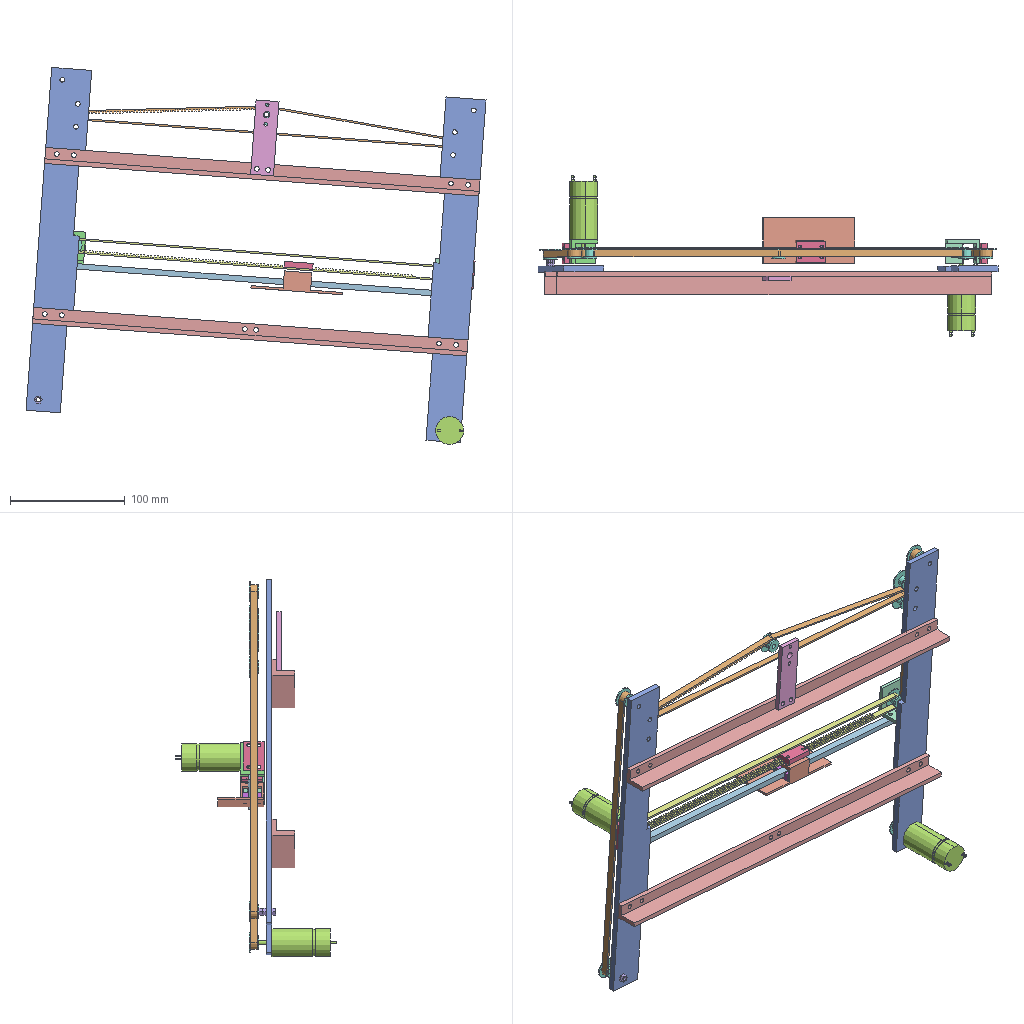Assembly | SolidWorks | 14 different items | 31 placed | box 401 x 140 x 329 mm
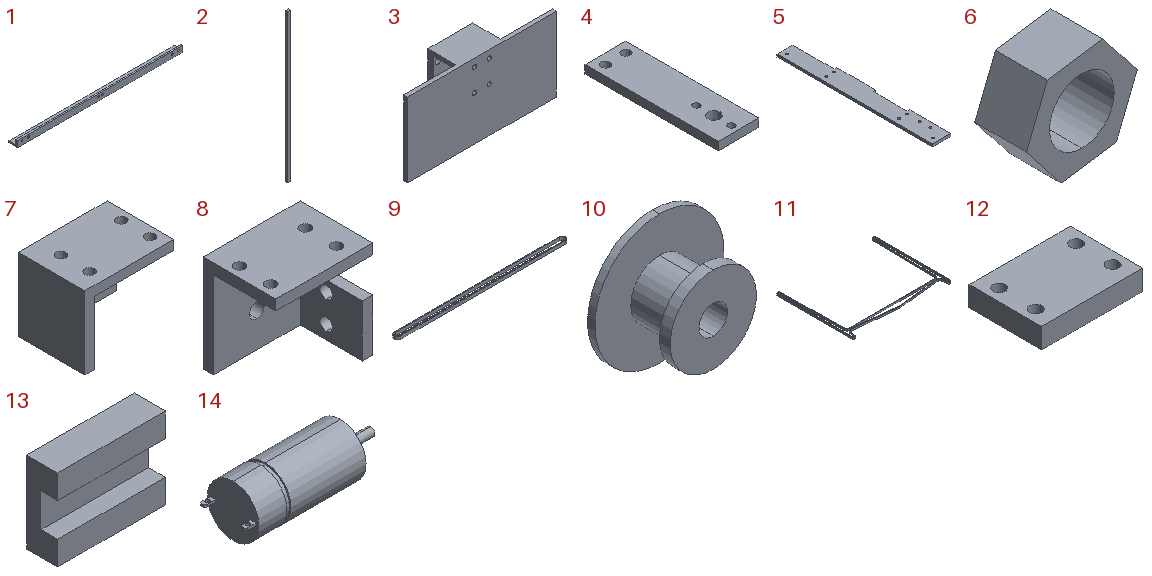Parts list (item | quantity | size | volume | features):
1 | x2 | 380 x 20 x 14 mm | 45267 mm3 | features Extrusion 1, ICE 1
2 | x1 | 7 x 4.8 x 340 mm | 11424 mm3 | features ICE 2, Extrusion 1, LPattern 1
3 | x1 | 80 x 17 x 40 mm | 8877 mm3 | features ICE 3, Extrusion 1
4 | x1 | 20 x 65 x 4 mm | 4912 mm3 | features Extrusion 1
5 | x2 | 35 x 300 x 5 mm | 48321 mm3 | features Extrusion 1
6 | x3 | 6.858 x 3.2 x 6.431 mm | 59.554 mm3 | features Extrusion 1
7 | x1 | 28 x 21 x 23 mm | 4355 mm3 | features ICE 2, Extrusion 1
8 | x1 | 28 x 21 x 28 mm | 4495 mm3 | features ICE 2, Extrusion 1
9 | x1 | 338 x 13 x 6 mm | 7437 mm3 | features Extrusion 1, ICE 1, LPattern 1
10 | x11 | 18 x 8.5 x 18 mm | 618.894 mm3 | features Revolution 1
11 | x1 | 372 x 292 x 6 mm | 17336 mm3 | features Extrusion 1, ICE 1, LPattern 1
12 | x3 | 25 x 18 x 5 mm | 2109 mm3 | features Extrusion 1
13 | x1 | 22.5 x 6.5 x 17 mm | 1885 mm3 | features Extrusion 1, ICE 1
14 | x2 | 70.5 x 24.5 x 24.5 mm | 24091 mm3 | features ICE 4, Extrusion 1, Fillet 1, RevCut 1
Mates (type | each side: item.copy, entity, surface, feature):
Concentric | 5.1 face cylinder Boss-Extrude1 | 10.1 face cylinder Revolve1
Concentric | 5.1 face cylinder Boss-Extrude1 | 10.2 face cylinder Revolve1
Concentric | 5.1 face cylinder Boss-Extrude1 | 10.3 face cylinder Revolve1
Concentric | 5.1 face cylinder Boss-Extrude1 | 10.4 face cylinder Revolve1
Coincident | 10.5 face plane Revolve1 | 10.3 face plane Revolve1
Concentric | 10.1 face cylinder Revolve1 | 11.1 face cylinder Boss-Extrude1
Concentric | 10.6 face cylinder Revolve1 | 11.1 face cylinder Boss-Extrude1
Coincident | 10.6 face plane Revolve1 | 11.1 face plane Boss-Extrude1
Concentric | 5.1 face cylinder Boss-Extrude1 | 6.1 face cylinder Boss-Extrude1
Coincident | 10.1 face plane Revolve1 | 6.1 face plane Boss-Extrude1
Coincident | 10.1 face plane Revolve1 | 11.1 face plane Boss-Extrude1
Coincident | 10.1 face plane Revolve1 | 10.4 face plane Revolve1
Coincident | 10.4 face plane Revolve1 | 10.3 face plane Revolve1
Coincident | 10.2 face plane Revolve1 | 10.4 face plane Revolve1
Coincident | 5.1 face plane Boss-Extrude1 | 6.2 face plane Boss-Extrude1
Coincident | 6.1 face plane Boss-Extrude1 | 6.3 face plane Boss-Extrude1
Coincident | 5.1 face plane Boss-Extrude1 | 6.3 face plane Boss-Extrude1
Coincident | 11.1 face plane Boss-Extrude1 | 12.1 face plane Boss-Extrude1
DistanceDim | 12.1 face plane Boss-Extrude1 | 11.1 face plane Boss-Extrude1
Coincident | 11.1 face plane Boss-Extrude1 | 8.1 face plane Boss-Extrude1
Concentric | 12.1 face cylinder Boss-Extrude1 | 8.1 face cylinder Boss-Extrude1 | 2 times
Concentric | 10.7 face cylinder Revolve1 | 8.1 face cylinder Boss-Extrude2
Parallel | 9.1 face plane Boss-Extrude1 | 8.1 face plane Boss-Extrude3
Concentric | 7.1 face cylinder Boss-Extrude2 | 10.8 face cylinder Revolve1
Coincident | 10.7 face plane Revolve1 | 9.1 face plane Boss-Extrude1
Coincident | 10.8 face plane Revolve1 | 9.1 face plane Boss-Extrude1
DistanceDim | 12.2 face plane Boss-Extrude1 | 7.1 face plane Boss-Extrude1
Concentric | 7.1 face cylinder Boss-Extrude1 | 12.2 face cylinder Boss-Extrude1 | 2 times
DistanceDim | 2.1 face plane Boss-Extrude1 | 7.1 face plane Boss-Extrude2
DistanceDim | 8.1 face plane Boss-Extrude2 | 2.1 face plane Boss-Extrude1
Coincident | 2.1 face plane Boss-Extrude1 | 8.1 face plane Boss-Extrude3 | 2 times
DistanceDim | 2.1 face plane Boss-Extrude1 | 7.1 face plane Boss-Extrude1
Coincident | 7.1 face plane Boss-Extrude3 | 2.1 face plane Boss-Extrude1
Coincident | 12.3 face plane Boss-Extrude1 | 9.1 face plane Boss-Extrude1
Coincident | 2.1 face plane Boss-Extrude1 | 13.1 face plane Boss-Extrude1 | 2 times
Coincident | 13.1 face plane Boss-Extrude1 | 3.1 face plane Boss-Extrude1
Concentric | 13.1 face cylinder Cut-Extrude1 | 3.1 face cylinder Boss-Extrude1 | 2 times
Concentric | 12.3 face cylinder Boss-Extrude1 | 3.1 face cylinder Cut-Extrude1 | 2 times
DistanceDim | 12.3 face plane Boss-Extrude1 | 9.1 face plane Boss-Extrude1
LimitDistanceDim | 3.1 face plane Boss-Extrude3 | 7.1 face plane Boss-Extrude2
LimitDistanceDim | 12.3 face plane Boss-Extrude1 | 1.1 face plane Boss-Extrude1
Concentric | 7.1 face cylinder Boss-Extrude2 | 14.1 face cylinder Boss-Extrude4
Coincident | 7.1 face plane Boss-Extrude2 | 14.1 face plane Boss-Extrude1
GearDim | 10.5 face cylinder Revolve1 | 10.9 face cylinder Revolve1
GearDim | 10.9 face cylinder Revolve1 | 10.10 face cylinder Revolve1
GearDim | 10.11 face cylinder Revolve1 | 10.6 face cylinder Revolve1
GearDim | 10.10 face cylinder Revolve1 | 10.6 face cylinder Revolve1
Concentric | 10.8 face cylinder Revolve1 | 9.1 face cylinder Boss-Extrude1
Coincident | 5.1 face plane Boss-Extrude1 | 5.2 face plane Boss-Extrude1 | 2 times
Coincident | 1.1 face plane Boss-Extrude1 | 5.2 face plane Boss-Extrude1
Concentric | 1.1 face cylinder Boss-Extrude1 | 5.2 face cylinder Boss-Extrude1
Concentric | 5.1 face cylinder Boss-Extrude1 | 1.1 face cylinder Boss-Extrude1
Coincident | 1.1 face plane Boss-Extrude2 | 4.1 face plane Boss-Extrude1
Concentric | 1.1 face cylinder Boss-Extrude1 | 4.1 face cylinder Boss-Extrude1
Coincident | 1.1 face plane Boss-Extrude1 | 4.1 face plane Boss-Extrude1
Concentric | 1.2 face cylinder Boss-Extrude1 | 5.2 face cylinder Boss-Extrude1 | 2 times
Coincident | 1.2 face plane Boss-Extrude1 | 5.1 face plane Boss-Extrude1
Concentric | 1.2 face cylinder Boss-Extrude1 | 5.1 face cylinder Boss-Extrude1
Concentric | 5.2 face cylinder Boss-Extrude1 | 14.2 face cylinder Boss-Extrude4
Coincident | 5.2 face plane Boss-Extrude1 | 14.2 face plane Boss-Extrude1
Concentric | 4.1 face cylinder Boss-Extrude1 | 10.5 face cylinder Revolve1